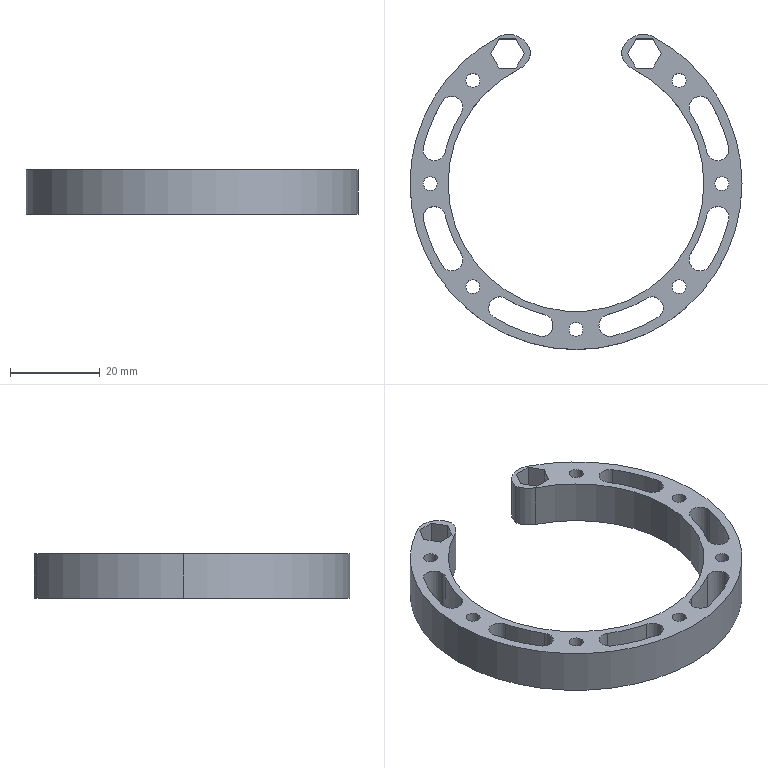Part | SolidWorks | features ICE 2, Extrusion 1, Fillet 1 | 1 solid | 68 faces | box 74 x 70.267 x 10 mm | volume 10018 mm3 | cylinder 54 | plane 14 | commonest cylinder face diameters 4.944 x18 3.1 x14 60.056 x6 69.944 x6 10 x4 57 x3